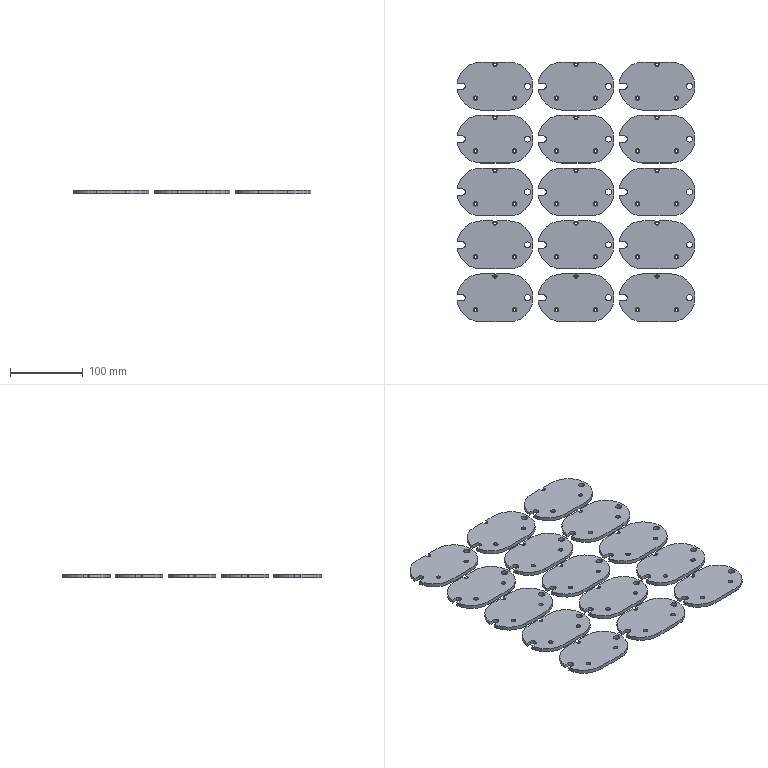Part | 15 solids | 330 faces | box 328.125 x 358 x 5 mm | volume 433676 mm3 | plane 165 | cylinder 165 | commonest cylinder face diameters 3.5 x45 6 x45 66 x45 8.5 x30